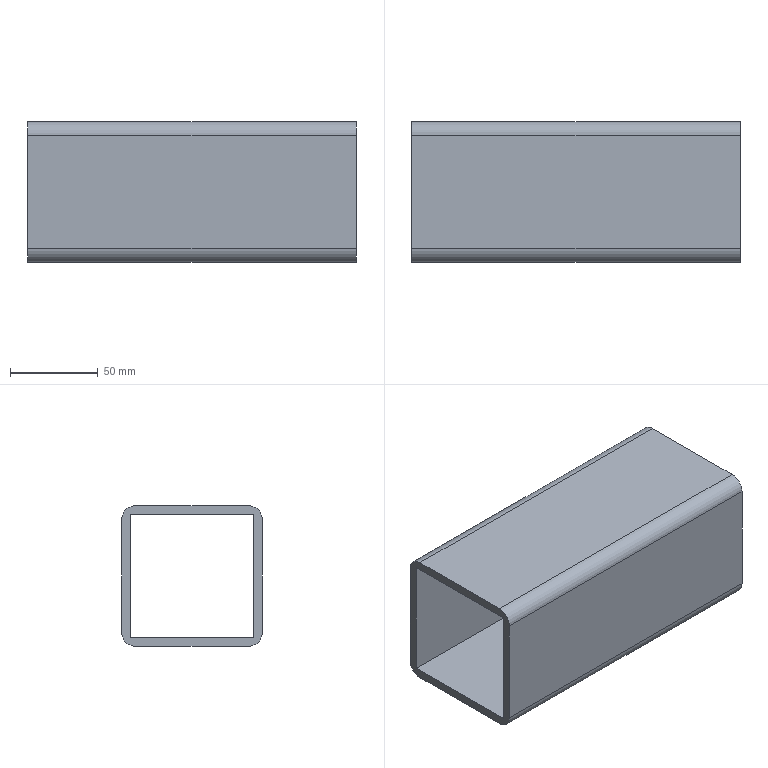Part | STEP file | Positioning_id970_x_t | 1 solid | 14 faces | box 187 x 80 x 80 mm | volume 270227 mm3 | plane 10 | cylinder 4 | commonest cylinder face diameters 16 x4
STEP:
#1=CARTESIAN_POINT('',(0.,0.,0.));
#2=DIRECTION('',(0.,0.,1.));
#3=DIRECTION('',(1.,0.,0.));
#4=AXIS2_PLACEMENT_3D('',#1,#2,#3);
#5=CARTESIAN_POINT('',(-808.002,-378.,258.995));
#6=VERTEX_POINT('',#5);
#7=CARTESIAN_POINT('',(-808.002,-370.,266.995));
#8=VERTEX_POINT('',#7);
#9=CARTESIAN_POINT('',(-808.002,-378.,266.995));
#10=DIRECTION('',(1.,0.,0.));
#11=DIRECTION('',(0.,1.,0.));
#12=AXIS2_PLACEMENT_3D('',#9,#10,#11);
#13=CIRCLE('',#12,8.);
#14=CARTESIAN_POINT('',(-925.002,-378.,266.995));
#15=DIRECTION('',(1.,0.,0.));
#16=DIRECTION('',(0.,0.,-1.));
#17=AXIS2_PLACEMENT_3D('',#14,#15,#16);
#18=CYLINDRICAL_SURFACE('',#17,8.);
#19=CARTESIAN_POINT('',(-4.712,117.));
#20=DIRECTION('',(1.,0.));
#21=VECTOR('',#20,1.);
#22=LINE('',#19,#21);
#23=(GEOMETRIC_REPRESENTATION_CONTEXT(2)PARAMETRIC_REPRESENTATION_CONTEXT()REPRESENTATION_CONTEXT('',''));
#24=DEFINITIONAL_REPRESENTATION('',(#22),#23);
#25=PCURVE('',#18,#24);
#26=CARTESIAN_POINT('',(-808.002,-410.,338.995));
#27=DIRECTION('',(1.,0.,0.));
#28=DIRECTION('',(0.,0.,-1.));
#29=AXIS2_PLACEMENT_3D('',#26,#27,#28);
#30=PLANE('',#29);
#31=CARTESIAN_POINT('',(72.,32.));
#32=DIRECTION('',(0.,1.));
#33=AXIS2_PLACEMENT_2D('',#31,#32);
#34=CIRCLE('',#33,8.);
#35=(GEOMETRIC_REPRESENTATION_CONTEXT(2)PARAMETRIC_REPRESENTATION_CONTEXT()REPRESENTATION_CONTEXT('',''));
#36=DEFINITIONAL_REPRESENTATION('',(#34),#35);
#37=PCURVE('',#30,#36);
#38=SURFACE_CURVE('',#13,(#25,#37),.PCURVE_S1.);
#39=EDGE_CURVE('',#6,#8,#38,.T.);
#40=ORIENTED_EDGE('',*,*,#39,.F.);
#41=CARTESIAN_POINT('',(-995.002,-378.,258.995));
#42=VERTEX_POINT('',#41);
#43=CARTESIAN_POINT('',(-995.002,-378.,258.995));
#44=DIRECTION('',(1.,0.,0.));
#45=VECTOR('',#44,1.);
#46=LINE('',#43,#45);
#47=CARTESIAN_POINT('',(0.,-70.));
#48=DIRECTION('',(0.,1.));
#49=VECTOR('',#48,1.);
#50=LINE('',#47,#49);
#51=(GEOMETRIC_REPRESENTATION_CONTEXT(2)PARAMETRIC_REPRESENTATION_CONTEXT()REPRESENTATION_CONTEXT('',''));
#52=DEFINITIONAL_REPRESENTATION('',(#50),#51);
#53=PCURVE('',#18,#52);
#54=CARTESIAN_POINT('',(-925.002,-410.,258.995));
#55=DIRECTION('',(0.,0.,-1.));
#56=DIRECTION('',(-1.,0.,0.));
#57=AXIS2_PLACEMENT_3D('',#54,#55,#56);
#58=PLANE('',#57);
#59=CARTESIAN_POINT('',(70.,32.));
#60=DIRECTION('',(-1.,0.));
#61=VECTOR('',#60,1.);
#62=LINE('',#59,#61);
#63=(GEOMETRIC_REPRESENTATION_CONTEXT(2)PARAMETRIC_REPRESENTATION_CONTEXT()REPRESENTATION_CONTEXT('',''));
#64=DEFINITIONAL_REPRESENTATION('',(#62),#63);
#65=PCURVE('',#58,#64);
#66=SURFACE_CURVE('',#46,(#53,#65),.PCURVE_S1.);
#67=EDGE_CURVE('',#42,#6,#66,.T.);
#68=ORIENTED_EDGE('',*,*,#67,.F.);
#69=CARTESIAN_POINT('',(-995.002,-370.,266.995));
#70=VERTEX_POINT('',#69);
#71=CARTESIAN_POINT('',(-995.002,-378.,266.995));
#72=DIRECTION('',(-1.,0.,0.));
#73=DIRECTION('',(0.,1.,0.));
#74=AXIS2_PLACEMENT_3D('',#71,#72,#73);
#75=CIRCLE('',#74,8.);
#76=CARTESIAN_POINT('',(1.571,-70.));
#77=DIRECTION('',(-1.,0.));
#78=VECTOR('',#77,1.);
#79=LINE('',#76,#78);
#80=(GEOMETRIC_REPRESENTATION_CONTEXT(2)PARAMETRIC_REPRESENTATION_CONTEXT()REPRESENTATION_CONTEXT('',''));
#81=DEFINITIONAL_REPRESENTATION('',(#79),#80);
#82=PCURVE('',#18,#81);
#83=CARTESIAN_POINT('',(-995.002,-410.,338.995));
#84=DIRECTION('',(-1.,0.,0.));
#85=DIRECTION('',(0.,0.,1.));
#86=AXIS2_PLACEMENT_3D('',#83,#84,#85);
#87=PLANE('',#86);
#88=CARTESIAN_POINT('',(-72.,32.));
#89=DIRECTION('',(0.,1.));
#90=AXIS2_PLACEMENT_2D('',#88,#89);
#91=CIRCLE('',#90,8.);
#92=(GEOMETRIC_REPRESENTATION_CONTEXT(2)PARAMETRIC_REPRESENTATION_CONTEXT()REPRESENTATION_CONTEXT('',''));
#93=DEFINITIONAL_REPRESENTATION('',(#91),#92);
#94=PCURVE('',#87,#93);
#95=SURFACE_CURVE('',#75,(#82,#94),.PCURVE_S1.);
#96=EDGE_CURVE('',#70,#42,#95,.T.);
#97=ORIENTED_EDGE('',*,*,#96,.F.);
#98=CARTESIAN_POINT('',(-808.002,-370.,266.995));
#99=DIRECTION('',(-1.,0.,0.));
#100=VECTOR('',#99,1.);
#101=LINE('',#98,#100);
#102=CARTESIAN_POINT('',(1.571,117.));
#103=DIRECTION('',(0.,-1.));
#104=VECTOR('',#103,1.);
#105=LINE('',#102,#104);
#106=(GEOMETRIC_REPRESENTATION_CONTEXT(2)PARAMETRIC_REPRESENTATION_CONTEXT()REPRESENTATION_CONTEXT('',''));
#107=DEFINITIONAL_REPRESENTATION('',(#105),#106);
#108=PCURVE('',#18,#107);
#109=CARTESIAN_POINT('',(-925.002,-370.,338.995));
#110=DIRECTION('',(0.,1.,0.));
#111=DIRECTION('',(0.,0.,-1.));
#112=AXIS2_PLACEMENT_3D('',#109,#110,#111);
#113=PLANE('',#112);
#114=CARTESIAN_POINT('',(72.,-117.));
#115=DIRECTION('',(0.,1.));
#116=VECTOR('',#115,1.);
#117=LINE('',#114,#116);
#118=(GEOMETRIC_REPRESENTATION_CONTEXT(2)PARAMETRIC_REPRESENTATION_CONTEXT()REPRESENTATION_CONTEXT('',''));
#119=DEFINITIONAL_REPRESENTATION('',(#117),#118);
#120=PCURVE('',#113,#119);
#121=SURFACE_CURVE('',#101,(#108,#120),.PCURVE_S1.);
#122=EDGE_CURVE('',#8,#70,#121,.T.);
#123=ORIENTED_EDGE('',*,*,#122,.F.);
#124=EDGE_LOOP('',(#40,#68,#97,#123));
#125=FACE_BOUND('',#124,.T.);
#126=ADVANCED_FACE('',(#125),#18,.T.);
#127=CARTESIAN_POINT('',(-808.002,-442.,338.995));
#128=VERTEX_POINT('',#127);
#129=CARTESIAN_POINT('',(-808.002,-450.,330.995));
#130=VERTEX_POINT('',#129);
#131=CARTESIAN_POINT('',(-808.002,-442.,330.995));
#132=DIRECTION('',(1.,0.,0.));
#133=DIRECTION('',(0.,1.,0.));
#134=AXIS2_PLACEMENT_3D('',#131,#132,#133);
#135=CIRCLE('',#134,8.);
#136=CARTESIAN_POINT('',(-925.002,-442.,330.995));
#137=DIRECTION('',(1.,0.,0.));
#138=DIRECTION('',(0.,0.,-1.));
#139=AXIS2_PLACEMENT_3D('',#136,#137,#138);
#140=CYLINDRICAL_SURFACE('',#139,8.);
#141=CARTESIAN_POINT('',(1.571,117.));
#142=DIRECTION('',(1.,0.));
#143=VECTOR('',#142,1.);
#144=LINE('',#141,#143);
#145=(GEOMETRIC_REPRESENTATION_CONTEXT(2)PARAMETRIC_REPRESENTATION_CONTEXT()REPRESENTATION_CONTEXT('',''));
#146=DEFINITIONAL_REPRESENTATION('',(#144),#145);
#147=PCURVE('',#140,#146);
#148=CARTESIAN_POINT('',(8.,-32.));
#149=DIRECTION('',(0.,1.));
#150=AXIS2_PLACEMENT_2D('',#148,#149);
#151=CIRCLE('',#150,8.);
#152=(GEOMETRIC_REPRESENTATION_CONTEXT(2)PARAMETRIC_REPRESENTATION_CONTEXT()REPRESENTATION_CONTEXT('',''));
#153=DEFINITIONAL_REPRESENTATION('',(#151),#152);
#154=PCURVE('',#30,#153);
#155=SURFACE_CURVE('',#135,(#147,#154),.PCURVE_S1.);
#156=EDGE_CURVE('',#128,#130,#155,.T.);
#157=ORIENTED_EDGE('',*,*,#156,.F.);
#158=CARTESIAN_POINT('',(-995.002,-442.,338.995));
#159=VERTEX_POINT('',#158);
#160=CARTESIAN_POINT('',(-995.002,-442.,338.995));
#161=DIRECTION('',(1.,0.,0.));
#162=VECTOR('',#161,1.);
#163=LINE('',#160,#162);
#164=CARTESIAN_POINT('',(3.142,-70.));
#165=DIRECTION('',(0.,1.));
#166=VECTOR('',#165,1.);
#167=LINE('',#164,#166);
#168=(GEOMETRIC_REPRESENTATION_CONTEXT(2)PARAMETRIC_REPRESENTATION_CONTEXT()REPRESENTATION_CONTEXT('',''));
#169=DEFINITIONAL_REPRESENTATION('',(#167),#168);
#170=PCURVE('',#140,#169);
#171=CARTESIAN_POINT('',(-925.002,-410.,338.995));
#172=DIRECTION('',(0.,0.,1.));
#173=DIRECTION('',(1.,0.,0.));
#174=AXIS2_PLACEMENT_3D('',#171,#172,#173);
#175=PLANE('',#174);
#176=CARTESIAN_POINT('',(-70.,-32.));
#177=DIRECTION('',(1.,0.));
#178=VECTOR('',#177,1.);
#179=LINE('',#176,#178);
#180=(GEOMETRIC_REPRESENTATION_CONTEXT(2)PARAMETRIC_REPRESENTATION_CONTEXT()REPRESENTATION_CONTEXT('',''));
#181=DEFINITIONAL_REPRESENTATION('',(#179),#180);
#182=PCURVE('',#175,#181);
#183=SURFACE_CURVE('',#163,(#170,#182),.PCURVE_S1.);
#184=EDGE_CURVE('',#159,#128,#183,.T.);
#185=ORIENTED_EDGE('',*,*,#184,.F.);
#186=CARTESIAN_POINT('',(-995.002,-450.,330.995));
#187=VERTEX_POINT('',#186);
#188=CARTESIAN_POINT('',(-995.002,-442.,330.995));
#189=DIRECTION('',(-1.,0.,0.));
#190=DIRECTION('',(0.,1.,0.));
#191=AXIS2_PLACEMENT_3D('',#188,#189,#190);
#192=CIRCLE('',#191,8.);
#193=CARTESIAN_POINT('',(7.854,-70.));
#194=DIRECTION('',(-1.,0.));
#195=VECTOR('',#194,1.);
#196=LINE('',#193,#195);
#197=(GEOMETRIC_REPRESENTATION_CONTEXT(2)PARAMETRIC_REPRESENTATION_CONTEXT()REPRESENTATION_CONTEXT('',''));
#198=DEFINITIONAL_REPRESENTATION('',(#196),#197);
#199=PCURVE('',#140,#198);
#200=CARTESIAN_POINT('',(-8.,-32.));
#201=DIRECTION('',(0.,1.));
#202=AXIS2_PLACEMENT_2D('',#200,#201);
#203=CIRCLE('',#202,8.);
#204=(GEOMETRIC_REPRESENTATION_CONTEXT(2)PARAMETRIC_REPRESENTATION_CONTEXT()REPRESENTATION_CONTEXT('',''));
#205=DEFINITIONAL_REPRESENTATION('',(#203),#204);
#206=PCURVE('',#87,#205);
#207=SURFACE_CURVE('',#192,(#199,#206),.PCURVE_S1.);
#208=EDGE_CURVE('',#187,#159,#207,.T.);
#209=ORIENTED_EDGE('',*,*,#208,.F.);
#210=CARTESIAN_POINT('',(-808.002,-450.,330.995));
#211=DIRECTION('',(-1.,0.,0.));
#212=VECTOR('',#211,1.);
#213=LINE('',#210,#212);
#214=CARTESIAN_POINT('',(4.712,117.));
#215=DIRECTION('',(0.,-1.));
#216=VECTOR('',#215,1.);
#217=LINE('',#214,#216);
#218=(GEOMETRIC_REPRESENTATION_CONTEXT(2)PARAMETRIC_REPRESENTATION_CONTEXT()REPRESENTATION_CONTEXT('',''));
#219=DEFINITIONAL_REPRESENTATION('',(#217),#218);
#220=PCURVE('',#140,#219);
#221=CARTESIAN_POINT('',(-925.002,-450.,338.995));
#222=DIRECTION('',(0.,-1.,0.));
#223=DIRECTION('',(0.,0.,1.));
#224=AXIS2_PLACEMENT_3D('',#221,#222,#223);
#225=PLANE('',#224);
#226=CARTESIAN_POINT('',(-8.,-117.));
#227=DIRECTION('',(0.,1.));
#228=VECTOR('',#227,1.);
#229=LINE('',#226,#228);
#230=(GEOMETRIC_REPRESENTATION_CONTEXT(2)PARAMETRIC_REPRESENTATION_CONTEXT()REPRESENTATION_CONTEXT('',''));
#231=DEFINITIONAL_REPRESENTATION('',(#229),#230);
#232=PCURVE('',#225,#231);
#233=SURFACE_CURVE('',#213,(#220,#232),.PCURVE_S1.);
#234=EDGE_CURVE('',#130,#187,#233,.T.);
#235=ORIENTED_EDGE('',*,*,#234,.F.);
#236=EDGE_LOOP('',(#157,#185,#209,#235));
#237=FACE_BOUND('',#236,.T.);
#238=ADVANCED_FACE('',(#237),#140,.T.);
#239=CARTESIAN_POINT('',(-995.002,-378.,338.995));
#240=VERTEX_POINT('',#239);
#241=CARTESIAN_POINT('',(-995.002,-370.,330.995));
#242=VERTEX_POINT('',#241);
#243=CARTESIAN_POINT('',(-995.002,-378.,330.995));
#244=DIRECTION('',(-1.,0.,0.));
#245=DIRECTION('',(0.,-1.,0.));
#246=AXIS2_PLACEMENT_3D('',#243,#244,#245);
#247=CIRCLE('',#246,8.);
#248=CARTESIAN_POINT('',(-925.002,-378.,330.995));
#249=DIRECTION('',(-1.,0.,0.));
#250=DIRECTION('',(0.,0.,1.));
#251=AXIS2_PLACEMENT_3D('',#248,#249,#250);
#252=CYLINDRICAL_SURFACE('',#251,8.);
#253=CARTESIAN_POINT('',(-1.571,70.));
#254=DIRECTION('',(1.,0.));
#255=VECTOR('',#254,1.);
#256=LINE('',#253,#255);
#257=(GEOMETRIC_REPRESENTATION_CONTEXT(2)PARAMETRIC_REPRESENTATION_CONTEXT()REPRESENTATION_CONTEXT('',''));
#258=DEFINITIONAL_REPRESENTATION('',(#256),#257);
#259=PCURVE('',#252,#258);
#260=CARTESIAN_POINT('',(-8.,32.));
#261=DIRECTION('',(0.,-1.));
#262=AXIS2_PLACEMENT_2D('',#260,#261);
#263=CIRCLE('',#262,8.);
#264=(GEOMETRIC_REPRESENTATION_CONTEXT(2)PARAMETRIC_REPRESENTATION_CONTEXT()REPRESENTATION_CONTEXT('',''));
#265=DEFINITIONAL_REPRESENTATION('',(#263),#264);
#266=PCURVE('',#87,#265);
#267=SURFACE_CURVE('',#247,(#259,#266),.PCURVE_S1.);
#268=EDGE_CURVE('',#240,#242,#267,.T.);
#269=ORIENTED_EDGE('',*,*,#268,.F.);
#270=CARTESIAN_POINT('',(-808.002,-378.,338.995));
#271=VERTEX_POINT('',#270);
#272=CARTESIAN_POINT('',(-808.002,-378.,338.995));
#273=DIRECTION('',(-1.,0.,0.));
#274=VECTOR('',#273,1.);
#275=LINE('',#272,#274);
#276=CARTESIAN_POINT('',(0.,-117.));
#277=DIRECTION('',(0.,1.));
#278=VECTOR('',#277,1.);
#279=LINE('',#276,#278);
#280=(GEOMETRIC_REPRESENTATION_CONTEXT(2)PARAMETRIC_REPRESENTATION_CONTEXT()REPRESENTATION_CONTEXT('',''));
#281=DEFINITIONAL_REPRESENTATION('',(#279),#280);
#282=PCURVE('',#252,#281);
#283=CARTESIAN_POINT('',(117.,32.));
#284=DIRECTION('',(-1.,0.));
#285=VECTOR('',#284,1.);
#286=LINE('',#283,#285);
#287=(GEOMETRIC_REPRESENTATION_CONTEXT(2)PARAMETRIC_REPRESENTATION_CONTEXT()REPRESENTATION_CONTEXT('',''));
#288=DEFINITIONAL_REPRESENTATION('',(#286),#287);
#289=PCURVE('',#175,#288);
#290=SURFACE_CURVE('',#275,(#282,#289),.PCURVE_S1.);
#291=EDGE_CURVE('',#271,#240,#290,.T.);
#292=ORIENTED_EDGE('',*,*,#291,.F.);
#293=CARTESIAN_POINT('',(-808.002,-370.,330.995));
#294=VERTEX_POINT('',#293);
#295=CARTESIAN_POINT('',(-808.002,-378.,330.995));
#296=DIRECTION('',(1.,0.,0.));
#297=DIRECTION('',(0.,-1.,0.));
#298=AXIS2_PLACEMENT_3D('',#295,#296,#297);
#299=CIRCLE('',#298,8.);
#300=CARTESIAN_POINT('',(4.712,-117.));
#301=DIRECTION('',(-1.,0.));
#302=VECTOR('',#301,1.);
#303=LINE('',#300,#302);
#304=(GEOMETRIC_REPRESENTATION_CONTEXT(2)PARAMETRIC_REPRESENTATION_CONTEXT()REPRESENTATION_CONTEXT('',''));
#305=DEFINITIONAL_REPRESENTATION('',(#303),#304);
#306=PCURVE('',#252,#305);
#307=CARTESIAN_POINT('',(8.,32.));
#308=DIRECTION('',(0.,-1.));
#309=AXIS2_PLACEMENT_2D('',#307,#308);
#310=CIRCLE('',#309,8.);
#311=(GEOMETRIC_REPRESENTATION_CONTEXT(2)PARAMETRIC_REPRESENTATION_CONTEXT()REPRESENTATION_CONTEXT('',''));
#312=DEFINITIONAL_REPRESENTATION('',(#310),#311);
#313=PCURVE('',#30,#312);
#314=SURFACE_CURVE('',#299,(#306,#313),.PCURVE_S1.);
#315=EDGE_CURVE('',#294,#271,#314,.T.);
#316=ORIENTED_EDGE('',*,*,#315,.F.);
#317=CARTESIAN_POINT('',(-995.002,-370.,330.995));
#318=DIRECTION('',(1.,0.,0.));
#319=VECTOR('',#318,1.);
#320=LINE('',#317,#319);
#321=CARTESIAN_POINT('',(1.571,70.));
#322=DIRECTION('',(0.,-1.));
#323=VECTOR('',#322,1.);
#324=LINE('',#321,#323);
#325=(GEOMETRIC_REPRESENTATION_CONTEXT(2)PARAMETRIC_REPRESENTATION_CONTEXT()REPRESENTATION_CONTEXT('',''));
#326=DEFINITIONAL_REPRESENTATION('',(#324),#325);
#327=PCURVE('',#252,#326);
#328=CARTESIAN_POINT('',(8.,70.));
#329=DIRECTION('',(0.,-1.));
#330=VECTOR('',#329,1.);
#331=LINE('',#328,#330);
#332=(GEOMETRIC_REPRESENTATION_CONTEXT(2)PARAMETRIC_REPRESENTATION_CONTEXT()REPRESENTATION_CONTEXT('',''));
#333=DEFINITIONAL_REPRESENTATION('',(#331),#332);
#334=PCURVE('',#113,#333);
#335=SURFACE_CURVE('',#320,(#327,#334),.PCURVE_S1.);
#336=EDGE_CURVE('',#242,#294,#335,.T.);
#337=ORIENTED_EDGE('',*,*,#336,.F.);
#338=EDGE_LOOP('',(#269,#292,#316,#337));
#339=FACE_BOUND('',#338,.T.);
#340=ADVANCED_FACE('',(#339),#252,.T.);
#341=CARTESIAN_POINT('',(-995.002,-442.,258.995));
#342=VERTEX_POINT('',#341);
#343=CARTESIAN_POINT('',(-995.002,-450.,266.995));
#344=VERTEX_POINT('',#343);
#345=CARTESIAN_POINT('',(-995.002,-442.,266.995));
#346=DIRECTION('',(-1.,0.,0.));
#347=DIRECTION('',(0.,-1.,0.));
#348=AXIS2_PLACEMENT_3D('',#345,#346,#347);
#349=CIRCLE('',#348,8.);
#350=CARTESIAN_POINT('',(-925.002,-442.,266.995));
#351=DIRECTION('',(-1.,0.,0.));
#352=DIRECTION('',(0.,0.,1.));
#353=AXIS2_PLACEMENT_3D('',#350,#351,#352);
#354=CYLINDRICAL_SURFACE('',#353,8.);
#355=CARTESIAN_POINT('',(-1.571,70.));
#356=DIRECTION('',(1.,0.));
#357=VECTOR('',#356,1.);
#358=LINE('',#355,#357);
#359=(GEOMETRIC_REPRESENTATION_CONTEXT(2)PARAMETRIC_REPRESENTATION_CONTEXT()REPRESENTATION_CONTEXT('',''));
#360=DEFINITIONAL_REPRESENTATION('',(#358),#359);
#361=PCURVE('',#354,#360);
#362=CARTESIAN_POINT('',(-72.,-32.));
#363=DIRECTION('',(0.,-1.));
#364=AXIS2_PLACEMENT_2D('',#362,#363);
#365=CIRCLE('',#364,8.);
#366=(GEOMETRIC_REPRESENTATION_CONTEXT(2)PARAMETRIC_REPRESENTATION_CONTEXT()REPRESENTATION_CONTEXT('',''));
#367=DEFINITIONAL_REPRESENTATION('',(#365),#366);
#368=PCURVE('',#87,#367);
#369=SURFACE_CURVE('',#349,(#361,#368),.PCURVE_S1.);
#370=EDGE_CURVE('',#342,#344,#369,.T.);
#371=ORIENTED_EDGE('',*,*,#370,.F.);
#372=CARTESIAN_POINT('',(-808.002,-442.,258.995));
#373=VERTEX_POINT('',#372);
#374=CARTESIAN_POINT('',(-808.002,-442.,258.995));
#375=DIRECTION('',(-1.,0.,0.));
#376=VECTOR('',#375,1.);
#377=LINE('',#374,#376);
#378=CARTESIAN_POINT('',(3.142,-117.));
#379=DIRECTION('',(0.,1.));
#380=VECTOR('',#379,1.);
#381=LINE('',#378,#380);
#382=(GEOMETRIC_REPRESENTATION_CONTEXT(2)PARAMETRIC_REPRESENTATION_CONTEXT()REPRESENTATION_CONTEXT('',''));
#383=DEFINITIONAL_REPRESENTATION('',(#381),#382);
#384=PCURVE('',#354,#383);
#385=CARTESIAN_POINT('',(-117.,-32.));
#386=DIRECTION('',(1.,0.));
#387=VECTOR('',#386,1.);
#388=LINE('',#385,#387);
#389=(GEOMETRIC_REPRESENTATION_CONTEXT(2)PARAMETRIC_REPRESENTATION_CONTEXT()REPRESENTATION_CONTEXT('',''));
#390=DEFINITIONAL_REPRESENTATION('',(#388),#389);
#391=PCURVE('',#58,#390);
#392=SURFACE_CURVE('',#377,(#384,#391),.PCURVE_S1.);
#393=EDGE_CURVE('',#373,#342,#392,.T.);
#394=ORIENTED_EDGE('',*,*,#393,.F.);
#395=CARTESIAN_POINT('',(-808.002,-450.,266.995));
#396=VERTEX_POINT('',#395);
#397=CARTESIAN_POINT('',(-808.002,-442.,266.995));
#398=DIRECTION('',(1.,0.,0.));
#399=DIRECTION('',(0.,-1.,0.));
#400=AXIS2_PLACEMENT_3D('',#397,#398,#399);
#401=CIRCLE('',#400,8.);
#402=CARTESIAN_POINT('',(4.712,-117.));
#403=DIRECTION('',(-1.,0.));
#404=VECTOR('',#403,1.);
#405=LINE('',#402,#404);
#406=(GEOMETRIC_REPRESENTATION_CONTEXT(2)PARAMETRIC_REPRESENTATION_CONTEXT()REPRESENTATION_CONTEXT('',''));
#407=DEFINITIONAL_REPRESENTATION('',(#405),#406);
#408=PCURVE('',#354,#407);
#409=CARTESIAN_POINT('',(72.,-32.));
#410=DIRECTION('',(0.,-1.));
#411=AXIS2_PLACEMENT_2D('',#409,#410);
#412=CIRCLE('',#411,8.);
#413=(GEOMETRIC_REPRESENTATION_CONTEXT(2)PARAMETRIC_REPRESENTATION_CONTEXT()REPRESENTATION_CONTEXT('',''));
#414=DEFINITIONAL_REPRESENTATION('',(#412),#413);
#415=PCURVE('',#30,#414);
#416=SURFACE_CURVE('',#401,(#408,#415),.PCURVE_S1.);
#417=EDGE_CURVE('',#396,#373,#416,.T.);
#418=ORIENTED_EDGE('',*,*,#417,.F.);
#419=CARTESIAN_POINT('',(-995.002,-450.,266.995));
#420=DIRECTION('',(1.,0.,0.));
#421=VECTOR('',#420,1.);
#422=LINE('',#419,#421);
#423=CARTESIAN_POINT('',(4.712,70.));
#424=DIRECTION('',(0.,-1.));
#425=VECTOR('',#424,1.);
#426=LINE('',#423,#425);
#427=(GEOMETRIC_REPRESENTATION_CONTEXT(2)PARAMETRIC_REPRESENTATION_CONTEXT()REPRESENTATION_CONTEXT('',''));
#428=DEFINITIONAL_REPRESENTATION('',(#426),#427);
#429=PCURVE('',#354,#428);
#430=CARTESIAN_POINT('',(-72.,70.));
#431=DIRECTION('',(0.,-1.));
#432=VECTOR('',#431,1.);
#433=LINE('',#430,#432);
#434=(GEOMETRIC_REPRESENTATION_CONTEXT(2)PARAMETRIC_REPRESENTATION_CONTEXT()REPRESENTATION_CONTEXT('',''));
#435=DEFINITIONAL_REPRESENTATION('',(#433),#434);
#436=PCURVE('',#225,#435);
#437=SURFACE_CURVE('',#422,(#429,#436),.PCURVE_S1.);
#438=EDGE_CURVE('',#344,#396,#437,.T.);
#439=ORIENTED_EDGE('',*,*,#438,.F.);
#440=EDGE_LOOP('',(#371,#394,#418,#439));
#441=FACE_BOUND('',#440,.T.);
#442=ADVANCED_FACE('',(#441),#354,.T.);
#443=CARTESIAN_POINT('',(-808.002,-375.,333.995));
#444=VERTEX_POINT('',#443);
#445=CARTESIAN_POINT('',(-808.002,-445.,333.995));
#446=VERTEX_POINT('',#445);
#447=CARTESIAN_POINT('',(-808.002,-375.,333.995));
#448=DIRECTION('',(0.,-1.,0.));
#449=VECTOR('',#448,1.);
#450=LINE('',#447,#449);
#451=CARTESIAN_POINT('',(-695.002,-410.,333.995));
#452=DIRECTION('',(0.,0.,1.));
#453=DIRECTION('',(1.,0.,0.));
#454=AXIS2_PLACEMENT_3D('',#451,#452,#453);
#455=PLANE('',#454);
#456=CARTESIAN_POINT('',(-113.,35.));
#457=DIRECTION('',(0.,-1.));
#458=VECTOR('',#457,1.);
#459=LINE('',#456,#458);
#460=(GEOMETRIC_REPRESENTATION_CONTEXT(2)PARAMETRIC_REPRESENTATION_CONTEXT()REPRESENTATION_CONTEXT('',''));
#461=DEFINITIONAL_REPRESENTATION('',(#459),#460);
#462=PCURVE('',#455,#461);
#463=CARTESIAN_POINT('',(5.,35.));
#464=DIRECTION('',(0.,-1.));
#465=VECTOR('',#464,1.);
#466=LINE('',#463,#465);
#467=(GEOMETRIC_REPRESENTATION_CONTEXT(2)PARAMETRIC_REPRESENTATION_CONTEXT()REPRESENTATION_CONTEXT('',''));
#468=DEFINITIONAL_REPRESENTATION('',(#466),#467);
#469=PCURVE('',#30,#468);
#470=SURFACE_CURVE('',#450,(#462,#469),.PCURVE_S1.);
#471=EDGE_CURVE('',#444,#446,#470,.T.);
#472=ORIENTED_EDGE('',*,*,#471,.T.);
#473=CARTESIAN_POINT('',(-995.002,-445.,333.995));
#474=VERTEX_POINT('',#473);
#475=CARTESIAN_POINT('',(-808.002,-445.,333.995));
#476=DIRECTION('',(-1.,0.,0.));
#477=VECTOR('',#476,1.);
#478=LINE('',#475,#477);
#479=CARTESIAN_POINT('',(-113.,-35.));
#480=DIRECTION('',(-1.,0.));
#481=VECTOR('',#480,1.);
#482=LINE('',#479,#481);
#483=(GEOMETRIC_REPRESENTATION_CONTEXT(2)PARAMETRIC_REPRESENTATION_CONTEXT()REPRESENTATION_CONTEXT('',''));
#484=DEFINITIONAL_REPRESENTATION('',(#482),#483);
#485=PCURVE('',#455,#484);
#486=CARTESIAN_POINT('',(-695.002,-445.,333.995));
#487=DIRECTION('',(0.,-1.,0.));
#488=DIRECTION('',(0.,0.,1.));
#489=AXIS2_PLACEMENT_3D('',#486,#487,#488);
#490=PLANE('',#489);
#491=CARTESIAN_POINT('',(0.,113.));
#492=DIRECTION('',(0.,1.));
#493=VECTOR('',#492,1.);
#494=LINE('',#491,#493);
#495=(GEOMETRIC_REPRESENTATION_CONTEXT(2)PARAMETRIC_REPRESENTATION_CONTEXT()REPRESENTATION_CONTEXT('',''));
#496=DEFINITIONAL_REPRESENTATION('',(#494),#495);
#497=PCURVE('',#490,#496);
#498=SURFACE_CURVE('',#478,(#485,#497),.PCURVE_S1.);
#499=EDGE_CURVE('',#446,#474,#498,.T.);
#500=ORIENTED_EDGE('',*,*,#499,.T.);
#501=CARTESIAN_POINT('',(-995.002,-375.,333.995));
#502=VERTEX_POINT('',#501);
#503=CARTESIAN_POINT('',(-995.002,-445.,333.995));
#504=DIRECTION('',(0.,1.,0.));
#505=VECTOR('',#504,1.);
#506=LINE('',#503,#505);
#507=CARTESIAN_POINT('',(-300.,-35.));
#508=DIRECTION('',(0.,1.));
#509=VECTOR('',#508,1.);
#510=LINE('',#507,#509);
#511=(GEOMETRIC_REPRESENTATION_CONTEXT(2)PARAMETRIC_REPRESENTATION_CONTEXT()REPRESENTATION_CONTEXT('',''));
#512=DEFINITIONAL_REPRESENTATION('',(#510),#511);
#513=PCURVE('',#455,#512);
#514=CARTESIAN_POINT('',(-5.,-35.));
#515=DIRECTION('',(0.,1.));
#516=VECTOR('',#515,1.);
#517=LINE('',#514,#516);
#518=(GEOMETRIC_REPRESENTATION_CONTEXT(2)PARAMETRIC_REPRESENTATION_CONTEXT()REPRESENTATION_CONTEXT('',''));
#519=DEFINITIONAL_REPRESENTATION('',(#517),#518);
#520=PCURVE('',#87,#519);
#521=SURFACE_CURVE('',#506,(#513,#520),.PCURVE_S1.);
#522=EDGE_CURVE('',#474,#502,#521,.T.);
#523=ORIENTED_EDGE('',*,*,#522,.T.);
#524=CARTESIAN_POINT('',(-995.002,-375.,333.995));
#525=DIRECTION('',(1.,0.,0.));
#526=VECTOR('',#525,1.);
#527=LINE('',#524,#526);
#528=CARTESIAN_POINT('',(-300.,35.));
#529=DIRECTION('',(1.,0.));
#530=VECTOR('',#529,1.);
#531=LINE('',#528,#530);
#532=(GEOMETRIC_REPRESENTATION_CONTEXT(2)PARAMETRIC_REPRESENTATION_CONTEXT()REPRESENTATION_CONTEXT('',''));
#533=DEFINITIONAL_REPRESENTATION('',(#531),#532);
#534=PCURVE('',#455,#533);
#535=CARTESIAN_POINT('',(-695.002,-375.,333.995));
#536=DIRECTION('',(0.,1.,0.));
#537=DIRECTION('',(0.,0.,-1.));
#538=AXIS2_PLACEMENT_3D('',#535,#536,#537);
#539=PLANE('',#538);
#540=CARTESIAN_POINT('',(0.,300.));
#541=DIRECTION('',(0.,-1.));
#542=VECTOR('',#541,1.);
#543=LINE('',#540,#542);
#544=(GEOMETRIC_REPRESENTATION_CONTEXT(2)PARAMETRIC_REPRESENTATION_CONTEXT()REPRESENTATION_CONTEXT('',''));
#545=DEFINITIONAL_REPRESENTATION('',(#543),#544);
#546=PCURVE('',#539,#545);
#547=SURFACE_CURVE('',#527,(#534,#546),.PCURVE_S1.);
#548=EDGE_CURVE('',#502,#444,#547,.T.);
#549=ORIENTED_EDGE('',*,*,#548,.T.);
#550=EDGE_LOOP('',(#472,#500,#523,#549));
#551=FACE_BOUND('',#550,.T.);
#552=ADVANCED_FACE('',(#551),#455,.F.);
#553=CARTESIAN_POINT('',(-808.002,-445.,263.995));
#554=VERTEX_POINT('',#553);
#555=CARTESIAN_POINT('',(-808.002,-445.,333.995));
#556=DIRECTION('',(0.,0.,-1.));
#557=VECTOR('',#556,1.);
#558=LINE('',#555,#557);
#559=CARTESIAN_POINT('',(0.,113.));
#560=DIRECTION('',(-1.,0.));
#561=VECTOR('',#560,1.);
#562=LINE('',#559,#561);
#563=(GEOMETRIC_REPRESENTATION_CONTEXT(2)PARAMETRIC_REPRESENTATION_CONTEXT()REPRESENTATION_CONTEXT('',''));
#564=DEFINITIONAL_REPRESENTATION('',(#562),#563);
#565=PCURVE('',#490,#564);
#566=CARTESIAN_POINT('',(5.,-35.));
#567=DIRECTION('',(1.,0.));
#568=VECTOR('',#567,1.);
#569=LINE('',#566,#568);
#570=(GEOMETRIC_REPRESENTATION_CONTEXT(2)PARAMETRIC_REPRESENTATION_CONTEXT()REPRESENTATION_CONTEXT('',''));
#571=DEFINITIONAL_REPRESENTATION('',(#569),#570);
#572=PCURVE('',#30,#571);
#573=SURFACE_CURVE('',#558,(#565,#572),.PCURVE_S1.);
#574=EDGE_CURVE('',#446,#554,#573,.T.);
#575=ORIENTED_EDGE('',*,*,#574,.T.);
#576=CARTESIAN_POINT('',(-995.002,-445.,263.995));
#577=VERTEX_POINT('',#576);
#578=CARTESIAN_POINT('',(-995.002,-445.,263.995));
#579=DIRECTION('',(1.,0.,0.));
#580=VECTOR('',#579,1.);
#581=LINE('',#578,#580);
#582=CARTESIAN_POINT('',(-70.,300.));
#583=DIRECTION('',(0.,-1.));
#584=VECTOR('',#583,1.);
#585=LINE('',#582,#584);
#586=(GEOMETRIC_REPRESENTATION_CONTEXT(2)PARAMETRIC_REPRESENTATION_CONTEXT()REPRESENTATION_CONTEXT('',''));
#587=DEFINITIONAL_REPRESENTATION('',(#585),#586);
#588=PCURVE('',#490,#587);
#589=CARTESIAN_POINT('',(-695.002,-410.,263.995));
#590=DIRECTION('',(0.,0.,-1.));
#591=DIRECTION('',(-1.,0.,0.));
#592=AXIS2_PLACEMENT_3D('',#589,#590,#591);
#593=PLANE('',#592);
#594=CARTESIAN_POINT('',(300.,-35.));
#595=DIRECTION('',(-1.,0.));
#596=VECTOR('',#595,1.);
#597=LINE('',#594,#596);
#598=(GEOMETRIC_REPRESENTATION_CONTEXT(2)PARAMETRIC_REPRESENTATION_CONTEXT()REPRESENTATION_CONTEXT('',''));
#599=DEFINITIONAL_REPRESENTATION('',(#597),#598);
#600=PCURVE('',#593,#599);
#601=SURFACE_CURVE('',#581,(#588,#600),.PCURVE_S1.);
#602=EDGE_CURVE('',#577,#554,#601,.T.);
#603=ORIENTED_EDGE('',*,*,#602,.F.);
#604=CARTESIAN_POINT('',(-995.002,-445.,333.995));
#605=DIRECTION('',(0.,0.,-1.));
#606=VECTOR('',#605,1.);
#607=LINE('',#604,#606);
#608=CARTESIAN_POINT('',(0.,300.));
#609=DIRECTION('',(-1.,0.));
#610=VECTOR('',#609,1.);
#611=LINE('',#608,#610);
#612=(GEOMETRIC_REPRESENTATION_CONTEXT(2)PARAMETRIC_REPRESENTATION_CONTEXT()REPRESENTATION_CONTEXT('',''));
#613=DEFINITIONAL_REPRESENTATION('',(#611),#612);
#614=PCURVE('',#490,#613);
#615=CARTESIAN_POINT('',(-5.,-35.));
#616=DIRECTION('',(-1.,0.));
#617=VECTOR('',#616,1.);
#618=LINE('',#615,#617);
#619=(GEOMETRIC_REPRESENTATION_CONTEXT(2)PARAMETRIC_REPRESENTATION_CONTEXT()REPRESENTATION_CONTEXT('',''));
#620=DEFINITIONAL_REPRESENTATION('',(#618),#619);
#621=PCURVE('',#87,#620);
#622=SURFACE_CURVE('',#607,(#614,#621),.PCURVE_S1.);
#623=EDGE_CURVE('',#474,#577,#622,.T.);
#624=ORIENTED_EDGE('',*,*,#623,.F.);
#625=ORIENTED_EDGE('',*,*,#499,.F.);
#626=EDGE_LOOP('',(#575,#603,#624,#625));
#627=FACE_BOUND('',#626,.T.);
#628=ADVANCED_FACE('',(#627),#490,.F.);
#629=CARTESIAN_POINT('',(-808.002,-375.,263.995));
#630=VERTEX_POINT('',#629);
#631=CARTESIAN_POINT('',(-808.002,-375.,263.995));
#632=DIRECTION('',(0.,0.,1.));
#633=VECTOR('',#632,1.);
#634=LINE('',#631,#633);
#635=CARTESIAN_POINT('',(70.,113.));
#636=DIRECTION('',(-1.,0.));
#637=VECTOR('',#636,1.);
#638=LINE('',#635,#637);
#639=(GEOMETRIC_REPRESENTATION_CONTEXT(2)PARAMETRIC_REPRESENTATION_CONTEXT()REPRESENTATION_CONTEXT('',''));
#640=DEFINITIONAL_REPRESENTATION('',(#638),#639);
#641=PCURVE('',#539,#640);
#642=CARTESIAN_POINT('',(75.,35.));
#643=DIRECTION('',(-1.,0.));
#644=VECTOR('',#643,1.);
#645=LINE('',#642,#644);
#646=(GEOMETRIC_REPRESENTATION_CONTEXT(2)PARAMETRIC_REPRESENTATION_CONTEXT()REPRESENTATION_CONTEXT('',''));
#647=DEFINITIONAL_REPRESENTATION('',(#645),#646);
#648=PCURVE('',#30,#647);
#649=SURFACE_CURVE('',#634,(#641,#648),.PCURVE_S1.);
#650=EDGE_CURVE('',#630,#444,#649,.T.);
#651=ORIENTED_EDGE('',*,*,#650,.T.);
#652=ORIENTED_EDGE('',*,*,#548,.F.);
#653=CARTESIAN_POINT('',(-995.002,-375.,263.995));
#654=VERTEX_POINT('',#653);
#655=CARTESIAN_POINT('',(-995.002,-375.,333.995));
#656=DIRECTION('',(0.,0.,-1.));
#657=VECTOR('',#656,1.);
#658=LINE('',#655,#657);
#659=CARTESIAN_POINT('',(0.,300.));
#660=DIRECTION('',(1.,0.));
#661=VECTOR('',#660,1.);
#662=LINE('',#659,#661);
#663=(GEOMETRIC_REPRESENTATION_CONTEXT(2)PARAMETRIC_REPRESENTATION_CONTEXT()REPRESENTATION_CONTEXT('',''));
#664=DEFINITIONAL_REPRESENTATION('',(#662),#663);
#665=PCURVE('',#539,#664);
#666=CARTESIAN_POINT('',(-5.,35.));
#667=DIRECTION('',(-1.,0.));
#668=VECTOR('',#667,1.);
#669=LINE('',#666,#668);
#670=(GEOMETRIC_REPRESENTATION_CONTEXT(2)PARAMETRIC_REPRESENTATION_CONTEXT()REPRESENTATION_CONTEXT('',''));
#671=DEFINITIONAL_REPRESENTATION('',(#669),#670);
#672=PCURVE('',#87,#671);
#673=SURFACE_CURVE('',#658,(#665,#672),.PCURVE_S1.);
#674=EDGE_CURVE('',#502,#654,#673,.T.);
#675=ORIENTED_EDGE('',*,*,#674,.T.);
#676=CARTESIAN_POINT('',(-808.002,-375.,263.995));
#677=DIRECTION('',(-1.,0.,0.));
#678=VECTOR('',#677,1.);
#679=LINE('',#676,#678);
#680=CARTESIAN_POINT('',(70.,113.));
#681=DIRECTION('',(0.,1.));
#682=VECTOR('',#681,1.);
#683=LINE('',#680,#682);
#684=(GEOMETRIC_REPRESENTATION_CONTEXT(2)PARAMETRIC_REPRESENTATION_CONTEXT()REPRESENTATION_CONTEXT('',''));
#685=DEFINITIONAL_REPRESENTATION('',(#683),#684);
#686=PCURVE('',#539,#685);
#687=CARTESIAN_POINT('',(113.,35.));
#688=DIRECTION('',(1.,0.));
#689=VECTOR('',#688,1.);
#690=LINE('',#687,#689);
#691=(GEOMETRIC_REPRESENTATION_CONTEXT(2)PARAMETRIC_REPRESENTATION_CONTEXT()REPRESENTATION_CONTEXT('',''));
#692=DEFINITIONAL_REPRESENTATION('',(#690),#691);
#693=PCURVE('',#593,#692);
#694=SURFACE_CURVE('',#679,(#686,#693),.PCURVE_S1.);
#695=EDGE_CURVE('',#630,#654,#694,.T.);
#696=ORIENTED_EDGE('',*,*,#695,.F.);
#697=EDGE_LOOP('',(#651,#652,#675,#696));
#698=FACE_BOUND('',#697,.T.);
#699=ADVANCED_FACE('',(#698),#539,.F.);
#700=CARTESIAN_POINT('',(-808.002,-445.,263.995));
#701=DIRECTION('',(0.,1.,0.));
#702=VECTOR('',#701,1.);
#703=LINE('',#700,#702);
#704=CARTESIAN_POINT('',(113.,-35.));
#705=DIRECTION('',(0.,1.));
#706=VECTOR('',#705,1.);
#707=LINE('',#704,#706);
#708=(GEOMETRIC_REPRESENTATION_CONTEXT(2)PARAMETRIC_REPRESENTATION_CONTEXT()REPRESENTATION_CONTEXT('',''));
#709=DEFINITIONAL_REPRESENTATION('',(#707),#708);
#710=PCURVE('',#593,#709);
#711=CARTESIAN_POINT('',(75.,-35.));
#712=DIRECTION('',(0.,1.));
#713=VECTOR('',#712,1.);
#714=LINE('',#711,#713);
#715=(GEOMETRIC_REPRESENTATION_CONTEXT(2)PARAMETRIC_REPRESENTATION_CONTEXT()REPRESENTATION_CONTEXT('',''));
#716=DEFINITIONAL_REPRESENTATION('',(#714),#715);
#717=PCURVE('',#30,#716);
#718=SURFACE_CURVE('',#703,(#710,#717),.PCURVE_S1.);
#719=EDGE_CURVE('',#554,#630,#718,.T.);
#720=ORIENTED_EDGE('',*,*,#719,.T.);
#721=ORIENTED_EDGE('',*,*,#695,.T.);
#722=CARTESIAN_POINT('',(-995.002,-375.,263.995));
#723=DIRECTION('',(0.,-1.,0.));
#724=VECTOR('',#723,1.);
#725=LINE('',#722,#724);
#726=CARTESIAN_POINT('',(300.,35.));
#727=DIRECTION('',(0.,-1.));
#728=VECTOR('',#727,1.);
#729=LINE('',#726,#728);
#730=(GEOMETRIC_REPRESENTATION_CONTEXT(2)PARAMETRIC_REPRESENTATION_CONTEXT()REPRESENTATION_CONTEXT('',''));
#731=DEFINITIONAL_REPRESENTATION('',(#729),#730);
#732=PCURVE('',#593,#731);
#733=CARTESIAN_POINT('',(-75.,35.));
#734=DIRECTION('',(0.,-1.));
#735=VECTOR('',#734,1.);
#736=LINE('',#733,#735);
#737=(GEOMETRIC_REPRESENTATION_CONTEXT(2)PARAMETRIC_REPRESENTATION_CONTEXT()REPRESENTATION_CONTEXT('',''));
#738=DEFINITIONAL_REPRESENTATION('',(#736),#737);
#739=PCURVE('',#87,#738);
#740=SURFACE_CURVE('',#725,(#732,#739),.PCURVE_S1.);
#741=EDGE_CURVE('',#654,#577,#740,.T.);
#742=ORIENTED_EDGE('',*,*,#741,.T.);
#743=ORIENTED_EDGE('',*,*,#602,.T.);
#744=EDGE_LOOP('',(#720,#721,#742,#743));
#745=FACE_BOUND('',#744,.T.);
#746=ADVANCED_FACE('',(#745),#593,.F.);
#747=ORIENTED_EDGE('',*,*,#719,.F.);
#748=ORIENTED_EDGE('',*,*,#574,.F.);
#749=ORIENTED_EDGE('',*,*,#471,.F.);
#750=ORIENTED_EDGE('',*,*,#650,.F.);
#751=EDGE_LOOP('',(#747,#748,#749,#750));
#752=FACE_BOUND('',#751,.T.);
#753=CARTESIAN_POINT('',(-808.002,-450.,330.995));
#754=DIRECTION('',(0.,0.,-1.));
#755=VECTOR('',#754,1.);
#756=LINE('',#753,#755);
#757=CARTESIAN_POINT('',(8.,-40.));
#758=DIRECTION('',(1.,0.));
#759=VECTOR('',#758,1.);
#760=LINE('',#757,#759);
#761=(GEOMETRIC_REPRESENTATION_CONTEXT(2)PARAMETRIC_REPRESENTATION_CONTEXT()REPRESENTATION_CONTEXT('',''));
#762=DEFINITIONAL_REPRESENTATION('',(#760),#761);
#763=PCURVE('',#30,#762);
#764=CARTESIAN_POINT('',(-8.,-117.));
#765=DIRECTION('',(-1.,0.));
#766=VECTOR('',#765,1.);
#767=LINE('',#764,#766);
#768=(GEOMETRIC_REPRESENTATION_CONTEXT(2)PARAMETRIC_REPRESENTATION_CONTEXT()REPRESENTATION_CONTEXT('',''));
#769=DEFINITIONAL_REPRESENTATION('',(#767),#768);
#770=PCURVE('',#225,#769);
#771=SURFACE_CURVE('',#756,(#763,#770),.PCURVE_S1.);
#772=EDGE_CURVE('',#130,#396,#771,.T.);
#773=ORIENTED_EDGE('',*,*,#772,.T.);
#774=ORIENTED_EDGE('',*,*,#417,.T.);
#775=CARTESIAN_POINT('',(-808.002,-442.,258.995));
#776=DIRECTION('',(0.,1.,0.));
#777=VECTOR('',#776,1.);
#778=LINE('',#775,#777);
#779=CARTESIAN_POINT('',(80.,-32.));
#780=DIRECTION('',(0.,1.));
#781=VECTOR('',#780,1.);
#782=LINE('',#779,#781);
#783=(GEOMETRIC_REPRESENTATION_CONTEXT(2)PARAMETRIC_REPRESENTATION_CONTEXT()REPRESENTATION_CONTEXT('',''));
#784=DEFINITIONAL_REPRESENTATION('',(#782),#783);
#785=PCURVE('',#30,#784);
#786=CARTESIAN_POINT('',(-117.,-32.));
#787=DIRECTION('',(0.,1.));
#788=VECTOR('',#787,1.);
#789=LINE('',#786,#788);
#790=(GEOMETRIC_REPRESENTATION_CONTEXT(2)PARAMETRIC_REPRESENTATION_CONTEXT()REPRESENTATION_CONTEXT('',''));
#791=DEFINITIONAL_REPRESENTATION('',(#789),#790);
#792=PCURVE('',#58,#791);
#793=SURFACE_CURVE('',#778,(#785,#792),.PCURVE_S1.);
#794=EDGE_CURVE('',#373,#6,#793,.T.);
#795=ORIENTED_EDGE('',*,*,#794,.T.);
#796=ORIENTED_EDGE('',*,*,#39,.T.);
#797=CARTESIAN_POINT('',(-808.002,-370.,330.995));
#798=DIRECTION('',(0.,0.,-1.));
#799=VECTOR('',#798,1.);
#800=LINE('',#797,#799);
#801=CARTESIAN_POINT('',(8.,40.));
#802=DIRECTION('',(1.,0.));
#803=VECTOR('',#802,1.);
#804=LINE('',#801,#803);
#805=(GEOMETRIC_REPRESENTATION_CONTEXT(2)PARAMETRIC_REPRESENTATION_CONTEXT()REPRESENTATION_CONTEXT('',''));
#806=DEFINITIONAL_REPRESENTATION('',(#804),#805);
#807=PCURVE('',#30,#806);
#808=CARTESIAN_POINT('',(8.,-117.));
#809=DIRECTION('',(1.,0.));
#810=VECTOR('',#809,1.);
#811=LINE('',#808,#810);
#812=(GEOMETRIC_REPRESENTATION_CONTEXT(2)PARAMETRIC_REPRESENTATION_CONTEXT()REPRESENTATION_CONTEXT('',''));
#813=DEFINITIONAL_REPRESENTATION('',(#811),#812);
#814=PCURVE('',#113,#813);
#815=SURFACE_CURVE('',#800,(#807,#814),.PCURVE_S1.);
#816=EDGE_CURVE('',#294,#8,#815,.T.);
#817=ORIENTED_EDGE('',*,*,#816,.F.);
#818=ORIENTED_EDGE('',*,*,#315,.T.);
#819=CARTESIAN_POINT('',(-808.002,-378.,338.995));
#820=DIRECTION('',(0.,-1.,0.));
#821=VECTOR('',#820,1.);
#822=LINE('',#819,#821);
#823=CARTESIAN_POINT('',(0.,32.));
#824=DIRECTION('',(0.,-1.));
#825=VECTOR('',#824,1.);
#826=LINE('',#823,#825);
#827=(GEOMETRIC_REPRESENTATION_CONTEXT(2)PARAMETRIC_REPRESENTATION_CONTEXT()REPRESENTATION_CONTEXT('',''));
#828=DEFINITIONAL_REPRESENTATION('',(#826),#827);
#829=PCURVE('',#30,#828);
#830=CARTESIAN_POINT('',(117.,32.));
#831=DIRECTION('',(0.,-1.));
#832=VECTOR('',#831,1.);
#833=LINE('',#830,#832);
#834=(GEOMETRIC_REPRESENTATION_CONTEXT(2)PARAMETRIC_REPRESENTATION_CONTEXT()REPRESENTATION_CONTEXT('',''));
#835=DEFINITIONAL_REPRESENTATION('',(#833),#834);
#836=PCURVE('',#175,#835);
#837=SURFACE_CURVE('',#822,(#829,#836),.PCURVE_S1.);
#838=EDGE_CURVE('',#271,#128,#837,.T.);
#839=ORIENTED_EDGE('',*,*,#838,.T.);
#840=ORIENTED_EDGE('',*,*,#156,.T.);
#841=EDGE_LOOP('',(#773,#774,#795,#796,#817,#818,#839,#840));
#842=FACE_BOUND('',#841,.T.);
#843=ADVANCED_FACE('',(#752,#842),#30,.T.);
#844=ORIENTED_EDGE('',*,*,#838,.F.);
#845=ORIENTED_EDGE('',*,*,#291,.T.);
#846=CARTESIAN_POINT('',(-995.002,-442.,338.995));
#847=DIRECTION('',(0.,1.,0.));
#848=VECTOR('',#847,1.);
#849=LINE('',#846,#848);
#850=CARTESIAN_POINT('',(-70.,-32.));
#851=DIRECTION('',(0.,1.));
#852=VECTOR('',#851,1.);
#853=LINE('',#850,#852);
#854=(GEOMETRIC_REPRESENTATION_CONTEXT(2)PARAMETRIC_REPRESENTATION_CONTEXT()REPRESENTATION_CONTEXT('',''));
#855=DEFINITIONAL_REPRESENTATION('',(#853),#854);
#856=PCURVE('',#175,#855);
#857=CARTESIAN_POINT('',(0.,-32.));
#858=DIRECTION('',(0.,1.));
#859=VECTOR('',#858,1.);
#860=LINE('',#857,#859);
#861=(GEOMETRIC_REPRESENTATION_CONTEXT(2)PARAMETRIC_REPRESENTATION_CONTEXT()REPRESENTATION_CONTEXT('',''));
#862=DEFINITIONAL_REPRESENTATION('',(#860),#861);
#863=PCURVE('',#87,#862);
#864=SURFACE_CURVE('',#849,(#856,#863),.PCURVE_S1.);
#865=EDGE_CURVE('',#159,#240,#864,.T.);
#866=ORIENTED_EDGE('',*,*,#865,.F.);
#867=ORIENTED_EDGE('',*,*,#184,.T.);
#868=EDGE_LOOP('',(#844,#845,#866,#867));
#869=FACE_BOUND('',#868,.T.);
#870=ADVANCED_FACE('',(#869),#175,.T.);
#871=CARTESIAN_POINT('',(-995.002,-450.,330.995));
#872=DIRECTION('',(0.,0.,-1.));
#873=VECTOR('',#872,1.);
#874=LINE('',#871,#873);
#875=CARTESIAN_POINT('',(-8.,70.));
#876=DIRECTION('',(-1.,0.));
#877=VECTOR('',#876,1.);
#878=LINE('',#875,#877);
#879=(GEOMETRIC_REPRESENTATION_CONTEXT(2)PARAMETRIC_REPRESENTATION_CONTEXT()REPRESENTATION_CONTEXT('',''));
#880=DEFINITIONAL_REPRESENTATION('',(#878),#879);
#881=PCURVE('',#225,#880);
#882=CARTESIAN_POINT('',(-8.,-40.));
#883=DIRECTION('',(-1.,0.));
#884=VECTOR('',#883,1.);
#885=LINE('',#882,#884);
#886=(GEOMETRIC_REPRESENTATION_CONTEXT(2)PARAMETRIC_REPRESENTATION_CONTEXT()REPRESENTATION_CONTEXT('',''));
#887=DEFINITIONAL_REPRESENTATION('',(#885),#886);
#888=PCURVE('',#87,#887);
#889=SURFACE_CURVE('',#874,(#881,#888),.PCURVE_S1.);
#890=EDGE_CURVE('',#187,#344,#889,.T.);
#891=ORIENTED_EDGE('',*,*,#890,.T.);
#892=ORIENTED_EDGE('',*,*,#438,.T.);
#893=ORIENTED_EDGE('',*,*,#772,.F.);
#894=ORIENTED_EDGE('',*,*,#234,.T.);
#895=EDGE_LOOP('',(#891,#892,#893,#894));
#896=FACE_BOUND('',#895,.T.);
#897=ADVANCED_FACE('',(#896),#225,.T.);
#898=ORIENTED_EDGE('',*,*,#741,.F.);
#899=ORIENTED_EDGE('',*,*,#674,.F.);
#900=ORIENTED_EDGE('',*,*,#522,.F.);
#901=ORIENTED_EDGE('',*,*,#623,.T.);
#902=EDGE_LOOP('',(#898,#899,#900,#901));
#903=FACE_BOUND('',#902,.T.);
#904=CARTESIAN_POINT('',(-995.002,-378.,258.995));
#905=DIRECTION('',(0.,-1.,0.));
#906=VECTOR('',#905,1.);
#907=LINE('',#904,#906);
#908=CARTESIAN_POINT('',(-80.,32.));
#909=DIRECTION('',(0.,-1.));
#910=VECTOR('',#909,1.);
#911=LINE('',#908,#910);
#912=(GEOMETRIC_REPRESENTATION_CONTEXT(2)PARAMETRIC_REPRESENTATION_CONTEXT()REPRESENTATION_CONTEXT('',''));
#913=DEFINITIONAL_REPRESENTATION('',(#911),#912);
#914=PCURVE('',#87,#913);
#915=CARTESIAN_POINT('',(70.,32.));
#916=DIRECTION('',(0.,-1.));
#917=VECTOR('',#916,1.);
#918=LINE('',#915,#917);
#919=(GEOMETRIC_REPRESENTATION_CONTEXT(2)PARAMETRIC_REPRESENTATION_CONTEXT()REPRESENTATION_CONTEXT('',''));
#920=DEFINITIONAL_REPRESENTATION('',(#918),#919);
#921=PCURVE('',#58,#920);
#922=SURFACE_CURVE('',#907,(#914,#921),.PCURVE_S1.);
#923=EDGE_CURVE('',#42,#342,#922,.T.);
#924=ORIENTED_EDGE('',*,*,#923,.T.);
#925=ORIENTED_EDGE('',*,*,#370,.T.);
#926=ORIENTED_EDGE('',*,*,#890,.F.);
#927=ORIENTED_EDGE('',*,*,#208,.T.);
#928=ORIENTED_EDGE('',*,*,#865,.T.);
#929=ORIENTED_EDGE('',*,*,#268,.T.);
#930=CARTESIAN_POINT('',(-995.002,-370.,330.995));
#931=DIRECTION('',(0.,0.,-1.));
#932=VECTOR('',#931,1.);
#933=LINE('',#930,#932);
#934=CARTESIAN_POINT('',(-8.,40.));
#935=DIRECTION('',(-1.,0.));
#936=VECTOR('',#935,1.);
#937=LINE('',#934,#936);
#938=(GEOMETRIC_REPRESENTATION_CONTEXT(2)PARAMETRIC_REPRESENTATION_CONTEXT()REPRESENTATION_CONTEXT('',''));
#939=DEFINITIONAL_REPRESENTATION('',(#937),#938);
#940=PCURVE('',#87,#939);
#941=CARTESIAN_POINT('',(8.,70.));
#942=DIRECTION('',(1.,0.));
#943=VECTOR('',#942,1.);
#944=LINE('',#941,#943);
#945=(GEOMETRIC_REPRESENTATION_CONTEXT(2)PARAMETRIC_REPRESENTATION_CONTEXT()REPRESENTATION_CONTEXT('',''));
#946=DEFINITIONAL_REPRESENTATION('',(#944),#945);
#947=PCURVE('',#113,#946);
#948=SURFACE_CURVE('',#933,(#940,#947),.PCURVE_S1.);
#949=EDGE_CURVE('',#242,#70,#948,.T.);
#950=ORIENTED_EDGE('',*,*,#949,.T.);
#951=ORIENTED_EDGE('',*,*,#96,.T.);
#952=EDGE_LOOP('',(#924,#925,#926,#927,#928,#929,#950,#951));
#953=FACE_BOUND('',#952,.T.);
#954=ADVANCED_FACE('',(#903,#953),#87,.T.);
#955=ORIENTED_EDGE('',*,*,#949,.F.);
#956=ORIENTED_EDGE('',*,*,#336,.T.);
#957=ORIENTED_EDGE('',*,*,#816,.T.);
#958=ORIENTED_EDGE('',*,*,#122,.T.);
#959=EDGE_LOOP('',(#955,#956,#957,#958));
#960=FACE_BOUND('',#959,.T.);
#961=ADVANCED_FACE('',(#960),#113,.T.);
#962=ORIENTED_EDGE('',*,*,#794,.F.);
#963=ORIENTED_EDGE('',*,*,#393,.T.);
#964=ORIENTED_EDGE('',*,*,#923,.F.);
#965=ORIENTED_EDGE('',*,*,#67,.T.);
#966=EDGE_LOOP('',(#962,#963,#964,#965));
#967=FACE_BOUND('',#966,.T.);
#968=ADVANCED_FACE('',(#967),#58,.T.);
#969=CLOSED_SHELL('',(#126,#238,#340,#442,#552,#628,#699,#746,#843,#870,#897,#954,#961,#968));
#970=MANIFOLD_SOLID_BREP('',#969);
#971=(LENGTH_UNIT()NAMED_UNIT(*)SI_UNIT(.MILLI.,.METRE.));
#972=UNCERTAINTY_MEASURE_WITH_UNIT(LENGTH_MEASURE(0.0000001),#971,'','');
#973=(NAMED_UNIT(*)PLANE_ANGLE_UNIT()SI_UNIT($,.RADIAN.));
#974=(NAMED_UNIT(*)SI_UNIT($,.STERADIAN.)SOLID_ANGLE_UNIT());
#975=(GEOMETRIC_REPRESENTATION_CONTEXT(3)GLOBAL_UNCERTAINTY_ASSIGNED_CONTEXT((#972))GLOBAL_UNIT_ASSIGNED_CONTEXT((#971,#973,#974))REPRESENTATION_CONTEXT('',''));
#976=ADVANCED_BREP_SHAPE_REPRESENTATION('',(#4,#970),#975);